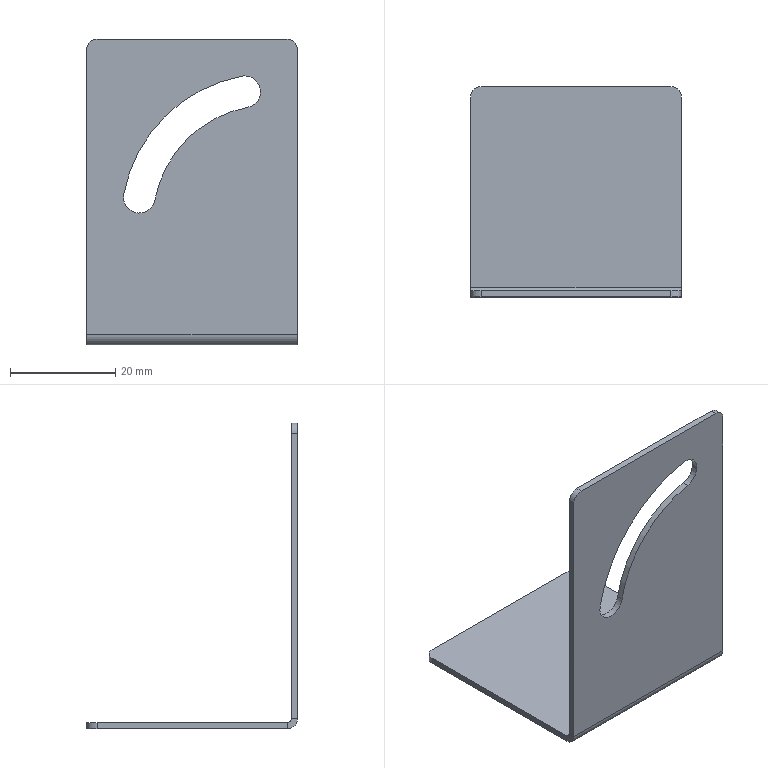Part | 1 solid | 23 faces | box 40 x 40 x 58 mm | volume 4364 mm3 | plane 12 | cylinder 11 | commonest cylinder face diameters 4 x4 6 x3 1.473 x1 3.873 x1 44 x1 56 x1
STEP:
#1=CARTESIAN_POINT('',(30.,0.,49.8));
#2=VERTEX_POINT('',#1);
#3=CARTESIAN_POINT('',(30.549,0.,43.851));
#4=VERTEX_POINT('',#3);
#5=CARTESIAN_POINT('',(30.,0.,46.8));
#6=DIRECTION('',(0.,1.,0.));
#7=DIRECTION('',(0.,0.,1.));
#8=AXIS2_PLACEMENT_3D('',#5,#6,#7);
#9=CIRCLE('',#8,3.);
#10=EDGE_CURVE('',#2,#4,#9,.T.);
#11=ORIENTED_EDGE('',*,*,#10,.F.);
#12=CARTESIAN_POINT('',(30.,1.2,49.8));
#13=VERTEX_POINT('',#12);
#14=CARTESIAN_POINT('',(30.,0.,49.8));
#15=DIRECTION('',(0.,1.,0.));
#16=VECTOR('',#15,1000.);
#17=LINE('',#14,#16);
#18=EDGE_CURVE('',#2,#13,#17,.T.);
#19=ORIENTED_EDGE('',*,*,#18,.T.);
#20=CARTESIAN_POINT('',(30.549,1.2,43.851));
#21=VERTEX_POINT('',#20);
#22=CARTESIAN_POINT('',(30.,1.2,46.8));
#23=DIRECTION('',(0.,1.,0.));
#24=DIRECTION('',(0.,0.,1.));
#25=AXIS2_PLACEMENT_3D('',#22,#23,#24);
#26=CIRCLE('',#25,3.);
#27=EDGE_CURVE('',#13,#21,#26,.T.);
#28=ORIENTED_EDGE('',*,*,#27,.T.);
#29=CARTESIAN_POINT('',(30.549,0.,43.851));
#30=DIRECTION('',(0.,1.,0.));
#31=VECTOR('',#30,1000.);
#32=LINE('',#29,#31);
#33=EDGE_CURVE('',#4,#21,#32,.T.);
#34=ORIENTED_EDGE('',*,*,#33,.F.);
#35=EDGE_LOOP('',(#11,#19,#28,#34));
#36=FACE_OUTER_BOUND('',#35,.T.);
#37=CARTESIAN_POINT('',(30.,0.,46.8));
#38=DIRECTION('',(0.,1.,0.));
#39=DIRECTION('',(0.,0.,1.));
#40=AXIS2_PLACEMENT_3D('',#37,#38,#39);
#41=CYLINDRICAL_SURFACE('',#40,3.);
#42=ADVANCED_FACE('',(#36),#41,.F.);
#43=CARTESIAN_POINT('',(40.,1.937,-1.2));
#44=VERTEX_POINT('',#43);
#45=CARTESIAN_POINT('',(40.,38.,-1.2));
#46=VERTEX_POINT('',#45);
#47=CARTESIAN_POINT('',(40.,0.,-1.2));
#48=DIRECTION('',(0.,1.,0.));
#49=VECTOR('',#48,1000.);
#50=LINE('',#47,#49);
#51=EDGE_CURVE('',#44,#46,#50,.T.);
#52=ORIENTED_EDGE('',*,*,#51,.T.);
#53=CARTESIAN_POINT('',(40.,38.,0.));
#54=VERTEX_POINT('',#53);
#55=CARTESIAN_POINT('',(40.,38.,-1.2));
#56=DIRECTION('',(0.,0.,1.));
#57=VECTOR('',#56,1000.);
#58=LINE('',#55,#57);
#59=EDGE_CURVE('',#46,#54,#58,.T.);
#60=ORIENTED_EDGE('',*,*,#59,.T.);
#61=CARTESIAN_POINT('',(40.,1.937,0.));
#62=VERTEX_POINT('',#61);
#63=CARTESIAN_POINT('',(40.,0.,0.));
#64=DIRECTION('',(0.,1.,0.));
#65=VECTOR('',#64,1000.);
#66=LINE('',#63,#65);
#67=EDGE_CURVE('',#62,#54,#66,.T.);
#68=ORIENTED_EDGE('',*,*,#67,.F.);
#69=CARTESIAN_POINT('',(40.,1.937,0.));
#70=DIRECTION('',(0.,0.,-1.));
#71=VECTOR('',#70,1000.);
#72=LINE('',#69,#71);
#73=EDGE_CURVE('',#62,#44,#72,.T.);
#74=ORIENTED_EDGE('',*,*,#73,.T.);
#75=EDGE_LOOP('',(#52,#60,#68,#74));
#76=FACE_OUTER_BOUND('',#75,.T.);
#77=CARTESIAN_POINT('',(40.,0.,-1.2));
#78=DIRECTION('',(1.,0.,0.));
#79=DIRECTION('',(0.,0.,-1.));
#80=AXIS2_PLACEMENT_3D('',#77,#78,#79);
#81=PLANE('',#80);
#82=ADVANCED_FACE('',(#76),#81,.T.);
#83=CARTESIAN_POINT('',(0.,38.,-1.2));
#84=VERTEX_POINT('',#83);
#85=CARTESIAN_POINT('',(0.,1.937,-1.2));
#86=VERTEX_POINT('',#85);
#87=CARTESIAN_POINT('',(0.,0.,-1.2));
#88=DIRECTION('',(0.,-1.,0.));
#89=VECTOR('',#88,1000.);
#90=LINE('',#87,#89);
#91=EDGE_CURVE('',#84,#86,#90,.T.);
#92=ORIENTED_EDGE('',*,*,#91,.F.);
#93=CARTESIAN_POINT('',(2.,40.,-1.2));
#94=VERTEX_POINT('',#93);
#95=CARTESIAN_POINT('',(2.,38.,-1.2));
#96=DIRECTION('',(0.,0.,-1.));
#97=DIRECTION('',(-1.,0.,0.));
#98=AXIS2_PLACEMENT_3D('',#95,#96,#97);
#99=CIRCLE('',#98,2.);
#100=EDGE_CURVE('',#84,#94,#99,.T.);
#101=ORIENTED_EDGE('',*,*,#100,.T.);
#102=CARTESIAN_POINT('',(38.,40.,-1.2));
#103=VERTEX_POINT('',#102);
#104=CARTESIAN_POINT('',(0.,40.,-1.2));
#105=DIRECTION('',(-1.,0.,0.));
#106=VECTOR('',#105,1000.);
#107=LINE('',#104,#106);
#108=EDGE_CURVE('',#103,#94,#107,.T.);
#109=ORIENTED_EDGE('',*,*,#108,.F.);
#110=CARTESIAN_POINT('',(38.,38.,-1.2));
#111=DIRECTION('',(0.,0.,-1.));
#112=DIRECTION('',(-1.,0.,0.));
#113=AXIS2_PLACEMENT_3D('',#110,#111,#112);
#114=CIRCLE('',#113,2.);
#115=EDGE_CURVE('',#103,#46,#114,.T.);
#116=ORIENTED_EDGE('',*,*,#115,.T.);
#117=ORIENTED_EDGE('',*,*,#51,.F.);
#118=CARTESIAN_POINT('',(40.,1.937,-1.2));
#119=DIRECTION('',(-1.,0.,0.));
#120=VECTOR('',#119,1000.);
#121=LINE('',#118,#120);
#122=EDGE_CURVE('',#44,#86,#121,.T.);
#123=ORIENTED_EDGE('',*,*,#122,.T.);
#124=EDGE_LOOP('',(#92,#101,#109,#116,#117,#123));
#125=FACE_OUTER_BOUND('',#124,.T.);
#126=CARTESIAN_POINT('',(0.,0.,-1.2));
#127=DIRECTION('',(0.,0.,-1.));
#128=DIRECTION('',(-1.,0.,0.));
#129=AXIS2_PLACEMENT_3D('',#126,#127,#128);
#130=PLANE('',#129);
#131=ADVANCED_FACE('',(#125),#130,.T.);
#132=CARTESIAN_POINT('',(38.,40.,0.));
#133=VERTEX_POINT('',#132);
#134=CARTESIAN_POINT('',(2.,40.,0.));
#135=VERTEX_POINT('',#134);
#136=CARTESIAN_POINT('',(0.,40.,0.));
#137=DIRECTION('',(-1.,0.,0.));
#138=VECTOR('',#137,1000.);
#139=LINE('',#136,#138);
#140=EDGE_CURVE('',#133,#135,#139,.T.);
#141=ORIENTED_EDGE('',*,*,#140,.T.);
#142=CARTESIAN_POINT('',(0.,38.,0.));
#143=VERTEX_POINT('',#142);
#144=CARTESIAN_POINT('',(2.,38.,0.));
#145=DIRECTION('',(0.,0.,1.));
#146=DIRECTION('',(-1.,0.,0.));
#147=AXIS2_PLACEMENT_3D('',#144,#145,#146);
#148=CIRCLE('',#147,2.);
#149=EDGE_CURVE('',#135,#143,#148,.T.);
#150=ORIENTED_EDGE('',*,*,#149,.T.);
#151=CARTESIAN_POINT('',(0.,1.937,0.));
#152=VERTEX_POINT('',#151);
#153=CARTESIAN_POINT('',(0.,0.,0.));
#154=DIRECTION('',(0.,-1.,0.));
#155=VECTOR('',#154,1000.);
#156=LINE('',#153,#155);
#157=EDGE_CURVE('',#143,#152,#156,.T.);
#158=ORIENTED_EDGE('',*,*,#157,.T.);
#159=CARTESIAN_POINT('',(40.,1.937,0.));
#160=DIRECTION('',(-1.,0.,0.));
#161=VECTOR('',#160,1000.);
#162=LINE('',#159,#161);
#163=EDGE_CURVE('',#62,#152,#162,.T.);
#164=ORIENTED_EDGE('',*,*,#163,.F.);
#165=ORIENTED_EDGE('',*,*,#67,.T.);
#166=CARTESIAN_POINT('',(38.,38.,0.));
#167=DIRECTION('',(0.,0.,1.));
#168=DIRECTION('',(-1.,0.,0.));
#169=AXIS2_PLACEMENT_3D('',#166,#167,#168);
#170=CIRCLE('',#169,2.);
#171=EDGE_CURVE('',#54,#133,#170,.T.);
#172=ORIENTED_EDGE('',*,*,#171,.T.);
#173=EDGE_LOOP('',(#141,#150,#158,#164,#165,#172));
#174=FACE_OUTER_BOUND('',#173,.T.);
#175=CARTESIAN_POINT('',(0.,0.,0.));
#176=DIRECTION('',(0.,0.,-1.));
#177=DIRECTION('',(-1.,0.,0.));
#178=AXIS2_PLACEMENT_3D('',#175,#176,#177);
#179=PLANE('',#178);
#180=ADVANCED_FACE('',(#174),#179,.F.);
#181=ORIENTED_EDGE('',*,*,#157,.F.);
#182=CARTESIAN_POINT('',(0.,38.,-1.2));
#183=DIRECTION('',(0.,0.,-1.));
#184=VECTOR('',#183,1000.);
#185=LINE('',#182,#184);
#186=EDGE_CURVE('',#143,#84,#185,.T.);
#187=ORIENTED_EDGE('',*,*,#186,.T.);
#188=ORIENTED_EDGE('',*,*,#91,.T.);
#189=CARTESIAN_POINT('',(0.,1.937,0.));
#190=DIRECTION('',(0.,0.,-1.));
#191=VECTOR('',#190,1000.);
#192=LINE('',#189,#191);
#193=EDGE_CURVE('',#152,#86,#192,.T.);
#194=ORIENTED_EDGE('',*,*,#193,.F.);
#195=EDGE_LOOP('',(#181,#187,#188,#194));
#196=FACE_OUTER_BOUND('',#195,.T.);
#197=CARTESIAN_POINT('',(0.,0.,-1.2));
#198=DIRECTION('',(-1.,0.,0.));
#199=DIRECTION('',(0.,0.,1.));
#200=AXIS2_PLACEMENT_3D('',#197,#198,#199);
#201=PLANE('',#200);
#202=ADVANCED_FACE('',(#196),#201,.T.);
#203=ORIENTED_EDGE('',*,*,#108,.T.);
#204=CARTESIAN_POINT('',(2.,40.,-1.2));
#205=DIRECTION('',(0.,0.,1.));
#206=VECTOR('',#205,1000.);
#207=LINE('',#204,#206);
#208=EDGE_CURVE('',#94,#135,#207,.T.);
#209=ORIENTED_EDGE('',*,*,#208,.T.);
#210=ORIENTED_EDGE('',*,*,#140,.F.);
#211=CARTESIAN_POINT('',(38.,40.,-1.2));
#212=DIRECTION('',(0.,0.,-1.));
#213=VECTOR('',#212,1000.);
#214=LINE('',#211,#213);
#215=EDGE_CURVE('',#133,#103,#214,.T.);
#216=ORIENTED_EDGE('',*,*,#215,.T.);
#217=EDGE_LOOP('',(#203,#209,#210,#216));
#218=FACE_OUTER_BOUND('',#217,.T.);
#219=CARTESIAN_POINT('',(0.,40.,-1.2));
#220=DIRECTION('',(0.,1.,0.));
#221=DIRECTION('',(0.,0.,1.));
#222=AXIS2_PLACEMENT_3D('',#219,#220,#221);
#223=PLANE('',#222);
#224=ADVANCED_FACE('',(#218),#223,.T.);
#225=CARTESIAN_POINT('',(0.,1.2,0.7366));
#226=VERTEX_POINT('',#225);
#227=CARTESIAN_POINT('',(0.,0.,0.7366));
#228=VERTEX_POINT('',#227);
#229=CARTESIAN_POINT('',(0.,0.,0.7366));
#230=DIRECTION('',(0.,-1.,0.));
#231=VECTOR('',#230,1000.);
#232=LINE('',#229,#231);
#233=EDGE_CURVE('',#226,#228,#232,.T.);
#234=ORIENTED_EDGE('',*,*,#233,.F.);
#235=CARTESIAN_POINT('',(0.,1.937,0.7366));
#236=DIRECTION('',(-1.,0.,0.));
#237=DIRECTION('',(0.,1.,0.));
#238=AXIS2_PLACEMENT_3D('',#235,#236,#237);
#239=CIRCLE('',#238,0.7366);
#240=EDGE_CURVE('',#152,#226,#239,.T.);
#241=ORIENTED_EDGE('',*,*,#240,.F.);
#242=ORIENTED_EDGE('',*,*,#193,.T.);
#243=CARTESIAN_POINT('',(0.,1.937,0.7366));
#244=DIRECTION('',(-1.,0.,0.));
#245=DIRECTION('',(0.,1.,0.));
#246=AXIS2_PLACEMENT_3D('',#243,#244,#245);
#247=CIRCLE('',#246,1.937);
#248=EDGE_CURVE('',#86,#228,#247,.T.);
#249=ORIENTED_EDGE('',*,*,#248,.T.);
#250=EDGE_LOOP('',(#234,#241,#242,#249));
#251=FACE_OUTER_BOUND('',#250,.T.);
#252=CARTESIAN_POINT('',(0.,1.937,0.7366));
#253=DIRECTION('',(-1.,0.,0.));
#254=DIRECTION('',(0.,-1.,0.));
#255=AXIS2_PLACEMENT_3D('',#252,#253,#254);
#256=PLANE('',#255);
#257=ADVANCED_FACE('',(#251),#256,.T.);
#258=CARTESIAN_POINT('',(40.,1.2,0.7366));
#259=VERTEX_POINT('',#258);
#260=CARTESIAN_POINT('',(40.,1.937,0.7366));
#261=DIRECTION('',(1.,0.,0.));
#262=DIRECTION('',(0.,1.,0.));
#263=AXIS2_PLACEMENT_3D('',#260,#261,#262);
#264=CIRCLE('',#263,0.7366);
#265=EDGE_CURVE('',#259,#62,#264,.T.);
#266=ORIENTED_EDGE('',*,*,#265,.F.);
#267=CARTESIAN_POINT('',(40.,0.,0.7366));
#268=VERTEX_POINT('',#267);
#269=CARTESIAN_POINT('',(40.,1.2,0.7366));
#270=DIRECTION('',(0.,-1.,0.));
#271=VECTOR('',#270,1000.);
#272=LINE('',#269,#271);
#273=EDGE_CURVE('',#259,#268,#272,.T.);
#274=ORIENTED_EDGE('',*,*,#273,.T.);
#275=CARTESIAN_POINT('',(40.,1.937,0.7366));
#276=DIRECTION('',(1.,0.,0.));
#277=DIRECTION('',(0.,1.,0.));
#278=AXIS2_PLACEMENT_3D('',#275,#276,#277);
#279=CIRCLE('',#278,1.937);
#280=EDGE_CURVE('',#268,#44,#279,.T.);
#281=ORIENTED_EDGE('',*,*,#280,.T.);
#282=ORIENTED_EDGE('',*,*,#73,.F.);
#283=EDGE_LOOP('',(#266,#274,#281,#282));
#284=FACE_OUTER_BOUND('',#283,.T.);
#285=CARTESIAN_POINT('',(40.,1.937,0.7366));
#286=DIRECTION('',(-1.,0.,0.));
#287=DIRECTION('',(0.,-1.,0.));
#288=AXIS2_PLACEMENT_3D('',#285,#286,#287);
#289=PLANE('',#288);
#290=ADVANCED_FACE('',(#284),#289,.F.);
#291=ORIENTED_EDGE('',*,*,#122,.F.);
#292=ORIENTED_EDGE('',*,*,#280,.F.);
#293=CARTESIAN_POINT('',(0.,0.,0.7366));
#294=DIRECTION('',(1.,0.,0.));
#295=VECTOR('',#294,1000.);
#296=LINE('',#293,#295);
#297=EDGE_CURVE('',#228,#268,#296,.T.);
#298=ORIENTED_EDGE('',*,*,#297,.F.);
#299=ORIENTED_EDGE('',*,*,#248,.F.);
#300=EDGE_LOOP('',(#291,#292,#298,#299));
#301=FACE_OUTER_BOUND('',#300,.T.);
#302=CARTESIAN_POINT('',(40.,1.937,0.7366));
#303=DIRECTION('',(1.,0.,0.));
#304=DIRECTION('',(0.,-1.,0.));
#305=AXIS2_PLACEMENT_3D('',#302,#303,#304);
#306=CYLINDRICAL_SURFACE('',#305,1.937);
#307=ADVANCED_FACE('',(#301),#306,.T.);
#308=ORIENTED_EDGE('',*,*,#163,.T.);
#309=ORIENTED_EDGE('',*,*,#240,.T.);
#310=CARTESIAN_POINT('',(0.,1.2,0.7366));
#311=DIRECTION('',(1.,0.,0.));
#312=VECTOR('',#311,1000.);
#313=LINE('',#310,#312);
#314=EDGE_CURVE('',#226,#259,#313,.T.);
#315=ORIENTED_EDGE('',*,*,#314,.T.);
#316=ORIENTED_EDGE('',*,*,#265,.T.);
#317=EDGE_LOOP('',(#308,#309,#315,#316));
#318=FACE_OUTER_BOUND('',#317,.T.);
#319=CARTESIAN_POINT('',(40.,1.937,0.7366));
#320=DIRECTION('',(1.,0.,0.));
#321=DIRECTION('',(0.,-1.,0.));
#322=AXIS2_PLACEMENT_3D('',#319,#320,#321);
#323=CYLINDRICAL_SURFACE('',#322,0.7366);
#324=ADVANCED_FACE('',(#318),#323,.F.);
#325=CARTESIAN_POINT('',(40.,1.2,54.8));
#326=VERTEX_POINT('',#325);
#327=CARTESIAN_POINT('',(40.,1.2,0.));
#328=DIRECTION('',(0.,0.,-1.));
#329=VECTOR('',#328,1000.);
#330=LINE('',#327,#329);
#331=EDGE_CURVE('',#326,#259,#330,.T.);
#332=ORIENTED_EDGE('',*,*,#331,.F.);
#333=CARTESIAN_POINT('',(40.,0.,54.8));
#334=VERTEX_POINT('',#333);
#335=CARTESIAN_POINT('',(40.,0.,54.8));
#336=DIRECTION('',(0.,-1.,0.));
#337=VECTOR('',#336,1000.);
#338=LINE('',#335,#337);
#339=EDGE_CURVE('',#326,#334,#338,.T.);
#340=ORIENTED_EDGE('',*,*,#339,.T.);
#341=CARTESIAN_POINT('',(40.,0.,0.));
#342=DIRECTION('',(0.,0.,-1.));
#343=VECTOR('',#342,1000.);
#344=LINE('',#341,#343);
#345=EDGE_CURVE('',#334,#268,#344,.T.);
#346=ORIENTED_EDGE('',*,*,#345,.T.);
#347=ORIENTED_EDGE('',*,*,#273,.F.);
#348=EDGE_LOOP('',(#332,#340,#346,#347));
#349=FACE_OUTER_BOUND('',#348,.T.);
#350=CARTESIAN_POINT('',(40.,0.,0.));
#351=DIRECTION('',(1.,0.,0.));
#352=DIRECTION('',(0.,0.,-1.));
#353=AXIS2_PLACEMENT_3D('',#350,#351,#352);
#354=PLANE('',#353);
#355=ADVANCED_FACE('',(#349),#354,.T.);
#356=CARTESIAN_POINT('',(0.,0.,54.8));
#357=VERTEX_POINT('',#356);
#358=CARTESIAN_POINT('',(0.,0.,56.8));
#359=DIRECTION('',(0.,0.,1.));
#360=VECTOR('',#359,1000.);
#361=LINE('',#358,#360);
#362=EDGE_CURVE('',#228,#357,#361,.T.);
#363=ORIENTED_EDGE('',*,*,#362,.T.);
#364=CARTESIAN_POINT('',(0.,1.2,54.8));
#365=VERTEX_POINT('',#364);
#366=CARTESIAN_POINT('',(0.,0.,54.8));
#367=DIRECTION('',(0.,1.,0.));
#368=VECTOR('',#367,1000.);
#369=LINE('',#366,#368);
#370=EDGE_CURVE('',#357,#365,#369,.T.);
#371=ORIENTED_EDGE('',*,*,#370,.T.);
#372=CARTESIAN_POINT('',(0.,1.2,0.));
#373=DIRECTION('',(0.,0.,1.));
#374=VECTOR('',#373,1000.);
#375=LINE('',#372,#374);
#376=EDGE_CURVE('',#226,#365,#375,.T.);
#377=ORIENTED_EDGE('',*,*,#376,.F.);
#378=ORIENTED_EDGE('',*,*,#233,.T.);
#379=EDGE_LOOP('',(#363,#371,#377,#378));
#380=FACE_OUTER_BOUND('',#379,.T.);
#381=CARTESIAN_POINT('',(0.,0.,56.8));
#382=DIRECTION('',(-1.,0.,0.));
#383=DIRECTION('',(0.,0.,1.));
#384=AXIS2_PLACEMENT_3D('',#381,#382,#383);
#385=PLANE('',#384);
#386=ADVANCED_FACE('',(#380),#385,.T.);
#387=CARTESIAN_POINT('',(12.949,0.,26.251));
#388=VERTEX_POINT('',#387);
#389=CARTESIAN_POINT('',(7.051,0.,27.349));
#390=VERTEX_POINT('',#389);
#391=CARTESIAN_POINT('',(10.,0.,26.8));
#392=DIRECTION('',(0.,1.,0.));
#393=DIRECTION('',(0.,0.,1.));
#394=AXIS2_PLACEMENT_3D('',#391,#392,#393);
#395=CIRCLE('',#394,3.);
#396=EDGE_CURVE('',#388,#390,#395,.T.);
#397=ORIENTED_EDGE('',*,*,#396,.T.);
#398=CARTESIAN_POINT('',(29.451,0.,49.749));
#399=VERTEX_POINT('',#398);
#400=CARTESIAN_POINT('',(34.577,0.,22.223));
#401=DIRECTION('',(0.,1.,0.));
#402=DIRECTION('',(0.,0.,1.));
#403=AXIS2_PLACEMENT_3D('',#400,#401,#402);
#404=CIRCLE('',#403,28.);
#405=EDGE_CURVE('',#390,#399,#404,.T.);
#406=ORIENTED_EDGE('',*,*,#405,.T.);
#407=CARTESIAN_POINT('',(30.,0.,46.8));
#408=DIRECTION('',(0.,1.,0.));
#409=DIRECTION('',(0.,0.,1.));
#410=AXIS2_PLACEMENT_3D('',#407,#408,#409);
#411=CIRCLE('',#410,3.);
#412=EDGE_CURVE('',#399,#2,#411,.T.);
#413=ORIENTED_EDGE('',*,*,#412,.T.);
#414=ORIENTED_EDGE('',*,*,#10,.T.);
#415=CARTESIAN_POINT('',(34.577,0.,22.223));
#416=DIRECTION('',(0.,-1.,0.));
#417=DIRECTION('',(0.,0.,1.));
#418=AXIS2_PLACEMENT_3D('',#415,#416,#417);
#419=CIRCLE('',#418,22.);
#420=EDGE_CURVE('',#4,#388,#419,.T.);
#421=ORIENTED_EDGE('',*,*,#420,.T.);
#422=EDGE_LOOP('',(#397,#406,#413,#414,#421));
#423=FACE_BOUND('',#422,.T.);
#424=ORIENTED_EDGE('',*,*,#345,.F.);
#425=CARTESIAN_POINT('',(38.,0.,56.8));
#426=VERTEX_POINT('',#425);
#427=CARTESIAN_POINT('',(38.,0.,54.8));
#428=DIRECTION('',(0.,-1.,0.));
#429=DIRECTION('',(0.,0.,-1.));
#430=AXIS2_PLACEMENT_3D('',#427,#428,#429);
#431=CIRCLE('',#430,2.);
#432=EDGE_CURVE('',#334,#426,#431,.T.);
#433=ORIENTED_EDGE('',*,*,#432,.T.);
#434=CARTESIAN_POINT('',(2.,0.,56.8));
#435=VERTEX_POINT('',#434);
#436=CARTESIAN_POINT('',(40.,0.,56.8));
#437=DIRECTION('',(1.,0.,0.));
#438=VECTOR('',#437,1000.);
#439=LINE('',#436,#438);
#440=EDGE_CURVE('',#435,#426,#439,.T.);
#441=ORIENTED_EDGE('',*,*,#440,.F.);
#442=CARTESIAN_POINT('',(2.,0.,54.8));
#443=DIRECTION('',(0.,-1.,0.));
#444=DIRECTION('',(0.,0.,-1.));
#445=AXIS2_PLACEMENT_3D('',#442,#443,#444);
#446=CIRCLE('',#445,2.);
#447=EDGE_CURVE('',#435,#357,#446,.T.);
#448=ORIENTED_EDGE('',*,*,#447,.T.);
#449=ORIENTED_EDGE('',*,*,#362,.F.);
#450=ORIENTED_EDGE('',*,*,#297,.T.);
#451=EDGE_LOOP('',(#424,#433,#441,#448,#449,#450));
#452=FACE_OUTER_BOUND('',#451,.T.);
#453=CARTESIAN_POINT('',(0.,0.,0.));
#454=DIRECTION('',(0.,-1.,0.));
#455=DIRECTION('',(0.,0.,-1.));
#456=AXIS2_PLACEMENT_3D('',#453,#454,#455);
#457=PLANE('',#456);
#458=ADVANCED_FACE('',(#423,#452),#457,.T.);
#459=CARTESIAN_POINT('',(7.051,1.2,27.349));
#460=VERTEX_POINT('',#459);
#461=CARTESIAN_POINT('',(29.451,1.2,49.749));
#462=VERTEX_POINT('',#461);
#463=CARTESIAN_POINT('',(34.577,1.2,22.223));
#464=DIRECTION('',(0.,1.,0.));
#465=DIRECTION('',(0.,0.,1.));
#466=AXIS2_PLACEMENT_3D('',#463,#464,#465);
#467=CIRCLE('',#466,28.);
#468=EDGE_CURVE('',#460,#462,#467,.T.);
#469=ORIENTED_EDGE('',*,*,#468,.F.);
#470=CARTESIAN_POINT('',(12.949,1.2,26.251));
#471=VERTEX_POINT('',#470);
#472=CARTESIAN_POINT('',(10.,1.2,26.8));
#473=DIRECTION('',(0.,1.,0.));
#474=DIRECTION('',(0.,0.,1.));
#475=AXIS2_PLACEMENT_3D('',#472,#473,#474);
#476=CIRCLE('',#475,3.);
#477=EDGE_CURVE('',#471,#460,#476,.T.);
#478=ORIENTED_EDGE('',*,*,#477,.F.);
#479=CARTESIAN_POINT('',(34.577,1.2,22.223));
#480=DIRECTION('',(0.,-1.,0.));
#481=DIRECTION('',(0.,0.,1.));
#482=AXIS2_PLACEMENT_3D('',#479,#480,#481);
#483=CIRCLE('',#482,22.);
#484=EDGE_CURVE('',#21,#471,#483,.T.);
#485=ORIENTED_EDGE('',*,*,#484,.F.);
#486=ORIENTED_EDGE('',*,*,#27,.F.);
#487=CARTESIAN_POINT('',(30.,1.2,46.8));
#488=DIRECTION('',(0.,1.,0.));
#489=DIRECTION('',(0.,0.,1.));
#490=AXIS2_PLACEMENT_3D('',#487,#488,#489);
#491=CIRCLE('',#490,3.);
#492=EDGE_CURVE('',#462,#13,#491,.T.);
#493=ORIENTED_EDGE('',*,*,#492,.F.);
#494=EDGE_LOOP('',(#469,#478,#485,#486,#493));
#495=FACE_BOUND('',#494,.T.);
#496=CARTESIAN_POINT('',(2.,1.2,56.8));
#497=VERTEX_POINT('',#496);
#498=CARTESIAN_POINT('',(38.,1.2,56.8));
#499=VERTEX_POINT('',#498);
#500=CARTESIAN_POINT('',(0.,1.2,56.8));
#501=DIRECTION('',(1.,0.,0.));
#502=VECTOR('',#501,1000.);
#503=LINE('',#500,#502);
#504=EDGE_CURVE('',#497,#499,#503,.T.);
#505=ORIENTED_EDGE('',*,*,#504,.T.);
#506=CARTESIAN_POINT('',(38.,1.2,54.8));
#507=DIRECTION('',(0.,1.,0.));
#508=DIRECTION('',(0.,0.,-1.));
#509=AXIS2_PLACEMENT_3D('',#506,#507,#508);
#510=CIRCLE('',#509,2.);
#511=EDGE_CURVE('',#499,#326,#510,.T.);
#512=ORIENTED_EDGE('',*,*,#511,.T.);
#513=ORIENTED_EDGE('',*,*,#331,.T.);
#514=ORIENTED_EDGE('',*,*,#314,.F.);
#515=ORIENTED_EDGE('',*,*,#376,.T.);
#516=CARTESIAN_POINT('',(2.,1.2,54.8));
#517=DIRECTION('',(0.,1.,0.));
#518=DIRECTION('',(0.,0.,-1.));
#519=AXIS2_PLACEMENT_3D('',#516,#517,#518);
#520=CIRCLE('',#519,2.);
#521=EDGE_CURVE('',#365,#497,#520,.T.);
#522=ORIENTED_EDGE('',*,*,#521,.T.);
#523=EDGE_LOOP('',(#505,#512,#513,#514,#515,#522));
#524=FACE_OUTER_BOUND('',#523,.T.);
#525=CARTESIAN_POINT('',(0.,1.2,0.));
#526=DIRECTION('',(0.,-1.,0.));
#527=DIRECTION('',(0.,0.,-1.));
#528=AXIS2_PLACEMENT_3D('',#525,#526,#527);
#529=PLANE('',#528);
#530=ADVANCED_FACE('',(#495,#524),#529,.F.);
#531=ORIENTED_EDGE('',*,*,#440,.T.);
#532=CARTESIAN_POINT('',(38.,0.,56.8));
#533=DIRECTION('',(0.,1.,0.));
#534=VECTOR('',#533,1000.);
#535=LINE('',#532,#534);
#536=EDGE_CURVE('',#426,#499,#535,.T.);
#537=ORIENTED_EDGE('',*,*,#536,.T.);
#538=ORIENTED_EDGE('',*,*,#504,.F.);
#539=CARTESIAN_POINT('',(2.,0.,56.8));
#540=DIRECTION('',(0.,-1.,0.));
#541=VECTOR('',#540,1000.);
#542=LINE('',#539,#541);
#543=EDGE_CURVE('',#497,#435,#542,.T.);
#544=ORIENTED_EDGE('',*,*,#543,.T.);
#545=EDGE_LOOP('',(#531,#537,#538,#544));
#546=FACE_OUTER_BOUND('',#545,.T.);
#547=CARTESIAN_POINT('',(40.,0.,56.8));
#548=DIRECTION('',(0.,0.,1.));
#549=DIRECTION('',(0.,-1.,0.));
#550=AXIS2_PLACEMENT_3D('',#547,#548,#549);
#551=PLANE('',#550);
#552=ADVANCED_FACE('',(#546),#551,.T.);
#553=ORIENTED_EDGE('',*,*,#477,.T.);
#554=CARTESIAN_POINT('',(7.051,0.,27.349));
#555=DIRECTION('',(0.,1.,0.));
#556=VECTOR('',#555,1000.);
#557=LINE('',#554,#556);
#558=EDGE_CURVE('',#390,#460,#557,.T.);
#559=ORIENTED_EDGE('',*,*,#558,.F.);
#560=ORIENTED_EDGE('',*,*,#396,.F.);
#561=CARTESIAN_POINT('',(12.949,0.,26.251));
#562=DIRECTION('',(0.,1.,0.));
#563=VECTOR('',#562,1000.);
#564=LINE('',#561,#563);
#565=EDGE_CURVE('',#388,#471,#564,.T.);
#566=ORIENTED_EDGE('',*,*,#565,.T.);
#567=EDGE_LOOP('',(#553,#559,#560,#566));
#568=FACE_OUTER_BOUND('',#567,.T.);
#569=CARTESIAN_POINT('',(10.,0.,26.8));
#570=DIRECTION('',(0.,1.,0.));
#571=DIRECTION('',(0.,0.,1.));
#572=AXIS2_PLACEMENT_3D('',#569,#570,#571);
#573=CYLINDRICAL_SURFACE('',#572,3.);
#574=ADVANCED_FACE('',(#568),#573,.F.);
#575=ORIENTED_EDGE('',*,*,#484,.T.);
#576=ORIENTED_EDGE('',*,*,#565,.F.);
#577=ORIENTED_EDGE('',*,*,#420,.F.);
#578=ORIENTED_EDGE('',*,*,#33,.T.);
#579=EDGE_LOOP('',(#575,#576,#577,#578));
#580=FACE_OUTER_BOUND('',#579,.T.);
#581=CARTESIAN_POINT('',(34.577,0.,22.223));
#582=DIRECTION('',(0.,1.,0.));
#583=DIRECTION('',(0.,0.,1.));
#584=AXIS2_PLACEMENT_3D('',#581,#582,#583);
#585=CYLINDRICAL_SURFACE('',#584,22.);
#586=ADVANCED_FACE('',(#580),#585,.T.);
#587=ORIENTED_EDGE('',*,*,#18,.F.);
#588=ORIENTED_EDGE('',*,*,#412,.F.);
#589=CARTESIAN_POINT('',(29.451,0.,49.749));
#590=DIRECTION('',(0.,1.,0.));
#591=VECTOR('',#590,1000.);
#592=LINE('',#589,#591);
#593=EDGE_CURVE('',#399,#462,#592,.T.);
#594=ORIENTED_EDGE('',*,*,#593,.T.);
#595=ORIENTED_EDGE('',*,*,#492,.T.);
#596=EDGE_LOOP('',(#587,#588,#594,#595));
#597=FACE_OUTER_BOUND('',#596,.T.);
#598=CARTESIAN_POINT('',(30.,0.,46.8));
#599=DIRECTION('',(0.,1.,0.));
#600=DIRECTION('',(0.,0.,1.));
#601=AXIS2_PLACEMENT_3D('',#598,#599,#600);
#602=CYLINDRICAL_SURFACE('',#601,3.);
#603=ADVANCED_FACE('',(#597),#602,.F.);
#604=ORIENTED_EDGE('',*,*,#468,.T.);
#605=ORIENTED_EDGE('',*,*,#593,.F.);
#606=ORIENTED_EDGE('',*,*,#405,.F.);
#607=ORIENTED_EDGE('',*,*,#558,.T.);
#608=EDGE_LOOP('',(#604,#605,#606,#607));
#609=FACE_OUTER_BOUND('',#608,.T.);
#610=CARTESIAN_POINT('',(34.577,0.,22.223));
#611=DIRECTION('',(0.,1.,0.));
#612=DIRECTION('',(0.,0.,1.));
#613=AXIS2_PLACEMENT_3D('',#610,#611,#612);
#614=CYLINDRICAL_SURFACE('',#613,28.);
#615=ADVANCED_FACE('',(#609),#614,.F.);
#616=ORIENTED_EDGE('',*,*,#432,.F.);
#617=ORIENTED_EDGE('',*,*,#339,.F.);
#618=ORIENTED_EDGE('',*,*,#511,.F.);
#619=ORIENTED_EDGE('',*,*,#536,.F.);
#620=EDGE_LOOP('',(#616,#617,#618,#619));
#621=FACE_OUTER_BOUND('',#620,.T.);
#622=CARTESIAN_POINT('',(38.,0.,54.8));
#623=DIRECTION('',(0.,1.,0.));
#624=DIRECTION('',(0.,0.,1.));
#625=AXIS2_PLACEMENT_3D('',#622,#623,#624);
#626=CYLINDRICAL_SURFACE('',#625,2.);
#627=ADVANCED_FACE('',(#621),#626,.T.);
#628=ORIENTED_EDGE('',*,*,#447,.F.);
#629=ORIENTED_EDGE('',*,*,#543,.F.);
#630=ORIENTED_EDGE('',*,*,#521,.F.);
#631=ORIENTED_EDGE('',*,*,#370,.F.);
#632=EDGE_LOOP('',(#628,#629,#630,#631));
#633=FACE_OUTER_BOUND('',#632,.T.);
#634=CARTESIAN_POINT('',(2.,0.,54.8));
#635=DIRECTION('',(0.,1.,0.));
#636=DIRECTION('',(0.,0.,1.));
#637=AXIS2_PLACEMENT_3D('',#634,#635,#636);
#638=CYLINDRICAL_SURFACE('',#637,2.);
#639=ADVANCED_FACE('',(#633),#638,.T.);
#640=ORIENTED_EDGE('',*,*,#100,.F.);
#641=ORIENTED_EDGE('',*,*,#186,.F.);
#642=ORIENTED_EDGE('',*,*,#149,.F.);
#643=ORIENTED_EDGE('',*,*,#208,.F.);
#644=EDGE_LOOP('',(#640,#641,#642,#643));
#645=FACE_OUTER_BOUND('',#644,.T.);
#646=CARTESIAN_POINT('',(2.,38.,-1.2));
#647=DIRECTION('',(0.,0.,1.));
#648=DIRECTION('',(1.,0.,0.));
#649=AXIS2_PLACEMENT_3D('',#646,#647,#648);
#650=CYLINDRICAL_SURFACE('',#649,2.);
#651=ADVANCED_FACE('',(#645),#650,.T.);
#652=ORIENTED_EDGE('',*,*,#115,.F.);
#653=ORIENTED_EDGE('',*,*,#215,.F.);
#654=ORIENTED_EDGE('',*,*,#171,.F.);
#655=ORIENTED_EDGE('',*,*,#59,.F.);
#656=EDGE_LOOP('',(#652,#653,#654,#655));
#657=FACE_OUTER_BOUND('',#656,.T.);
#658=CARTESIAN_POINT('',(38.,38.,-1.2));
#659=DIRECTION('',(0.,0.,1.));
#660=DIRECTION('',(1.,0.,0.));
#661=AXIS2_PLACEMENT_3D('',#658,#659,#660);
#662=CYLINDRICAL_SURFACE('',#661,2.);
#663=ADVANCED_FACE('',(#657),#662,.T.);
#664=CLOSED_SHELL('',(#42,#82,#131,#180,#202,#224,#257,#290,#307,#324,#355,#386,#458,#530,#552,#574,#586,#603,#615,#627,#639,#651,#663));
#665=MANIFOLD_SOLID_BREP('',#664);
#666=CARTESIAN_POINT('',(0.,0.,0.));
#667=DIRECTION('',(0.,0.,1.));
#668=DIRECTION('',(1.,0.,0.));
#669=AXIS2_PLACEMENT_3D('',#666,#667,#668);
#670=(LENGTH_UNIT()NAMED_UNIT(*)SI_UNIT(.MILLI.,.METRE.));
#671=UNCERTAINTY_MEASURE_WITH_UNIT(LENGTH_MEASURE(0.00001),#670,'','');
#672=(NAMED_UNIT(*)PLANE_ANGLE_UNIT()SI_UNIT($,.RADIAN.));
#673=(NAMED_UNIT(*)SI_UNIT($,.STERADIAN.)SOLID_ANGLE_UNIT());
#674=(GEOMETRIC_REPRESENTATION_CONTEXT(3)GLOBAL_UNCERTAINTY_ASSIGNED_CONTEXT((#671))GLOBAL_UNIT_ASSIGNED_CONTEXT((#670,#672,#673))REPRESENTATION_CONTEXT('',''));
#675=ADVANCED_BREP_SHAPE_REPRESENTATION('',(#665,#669),#674);